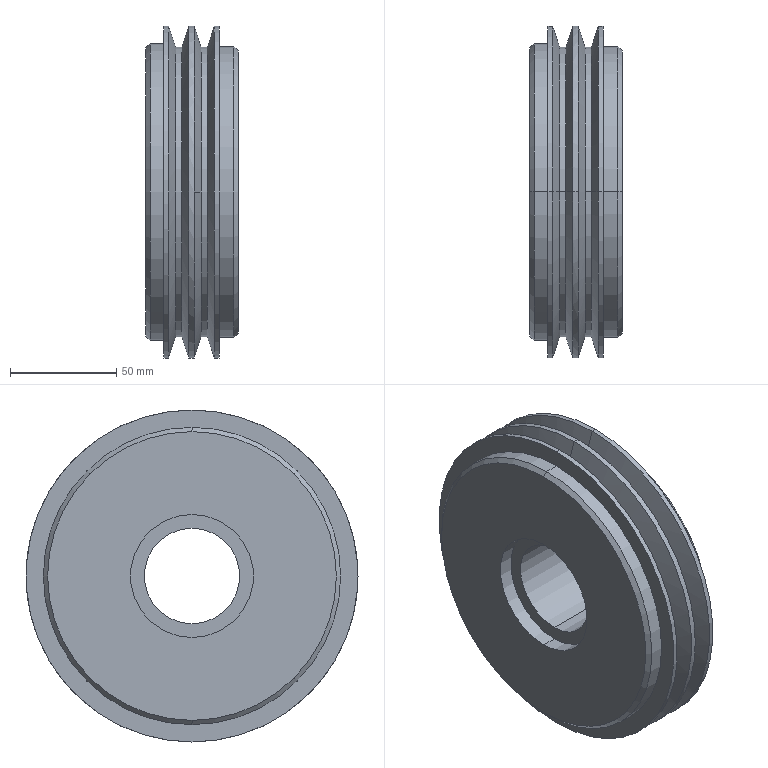Part | STEP file | 10P30 rotor 2 | 1 solid | 41 faces | box 43.5 x 156.4 x 156.4 mm | volume 346928 mm3 | cylinder 22 | cone 12 | plane 7 | commonest cylinder face diameters 156.4 x6 136.4 x4 45 x2 58 x2 85 x2 129.8 x2